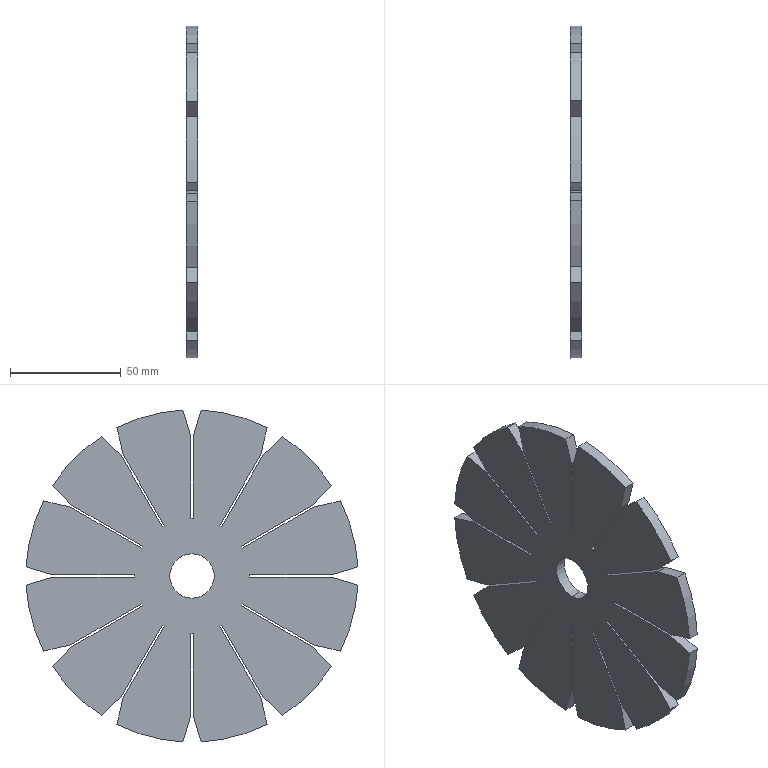Part | SolidWorks | features BaseBody 1 | 1 solid | 76 faces | box 5 x 149.779 x 149.779 mm | volume 81255 mm3 | plane 62 | cylinder 14 | commonest cylinder face diameters 150 x12 20 x2